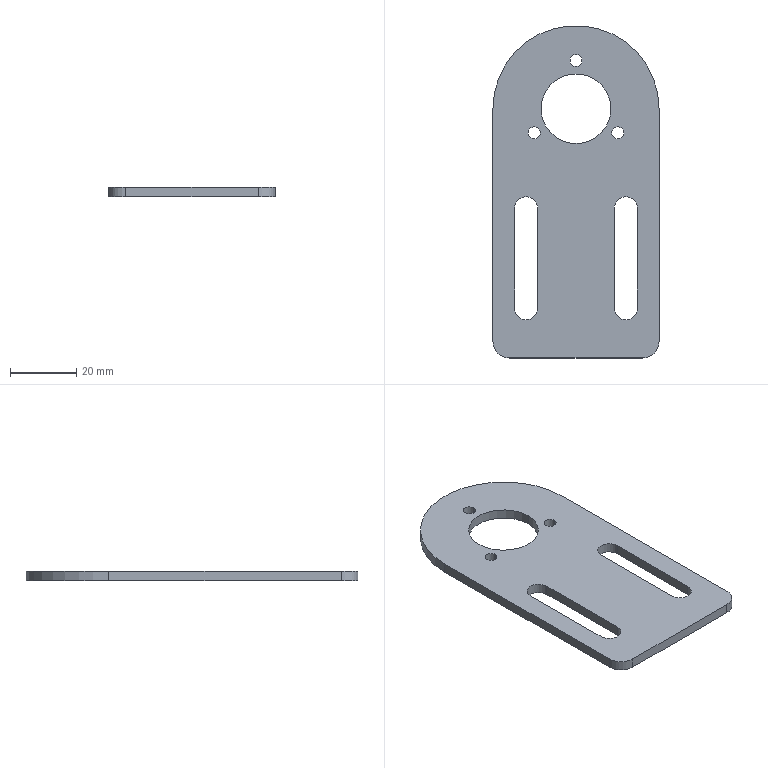Part | SolidWorks | features ICE 2, Fillet 1, FlatPattern 1, HoleWzd 1, SMBaseFlange 1, SheetMetal 1 | 1 solid | 24 faces | box 50 x 100 x 3 mm | volume 11541 mm3 | cylinder 15 | plane 9 | commonest cylinder face diameters 3.6 x6 7 x4 10 x2 21 x2 50 x1
STEP:
#1=CARTESIAN_POINT('',(23.2,89.5,-3.));
#2=VERTEX_POINT('',#1);
#3=CARTESIAN_POINT('',(26.8,89.5,-3.));
#4=VERTEX_POINT('',#3);
#5=CARTESIAN_POINT('',(25.,89.5,-3.));
#6=DIRECTION('',(0.,0.,1.));
#7=DIRECTION('',(1.,0.,0.));
#8=AXIS2_PLACEMENT_3D('',#5,#6,#7);
#9=CIRCLE('',#8,1.8);
#10=EDGE_CURVE('',#2,#4,#9,.T.);
#11=ORIENTED_EDGE('',*,*,#10,.F.);
#12=CARTESIAN_POINT('',(23.2,89.5,0.));
#13=VERTEX_POINT('',#12);
#14=CARTESIAN_POINT('',(23.2,89.5,0.));
#15=DIRECTION('',(0.,0.,1.));
#16=VECTOR('',#15,1000.);
#17=LINE('',#14,#16);
#18=EDGE_CURVE('',#2,#13,#17,.T.);
#19=ORIENTED_EDGE('',*,*,#18,.T.);
#20=CARTESIAN_POINT('',(26.8,89.5,0.));
#21=VERTEX_POINT('',#20);
#22=CARTESIAN_POINT('',(25.,89.5,0.));
#23=DIRECTION('',(0.,0.,1.));
#24=DIRECTION('',(1.,0.,0.));
#25=AXIS2_PLACEMENT_3D('',#22,#23,#24);
#26=CIRCLE('',#25,1.8);
#27=EDGE_CURVE('',#13,#21,#26,.T.);
#28=ORIENTED_EDGE('',*,*,#27,.T.);
#29=CARTESIAN_POINT('',(26.8,89.5,0.));
#30=DIRECTION('',(0.,0.,1.));
#31=VECTOR('',#30,1000.);
#32=LINE('',#29,#31);
#33=EDGE_CURVE('',#4,#21,#32,.T.);
#34=ORIENTED_EDGE('',*,*,#33,.F.);
#35=EDGE_LOOP('',(#11,#19,#28,#34));
#36=FACE_OUTER_BOUND('',#35,.T.);
#37=CARTESIAN_POINT('',(25.,89.5,0.));
#38=DIRECTION('',(0.,0.,1.));
#39=DIRECTION('',(1.,0.,0.));
#40=AXIS2_PLACEMENT_3D('',#37,#38,#39);
#41=CYLINDRICAL_SURFACE('',#40,1.8);
#42=ADVANCED_FACE('',(#36),#41,.F.);
#43=CARTESIAN_POINT('',(10.643,67.75,-3.));
#44=VERTEX_POINT('',#43);
#45=CARTESIAN_POINT('',(14.243,67.75,-3.));
#46=VERTEX_POINT('',#45);
#47=CARTESIAN_POINT('',(12.443,67.75,-3.));
#48=DIRECTION('',(0.,0.,1.));
#49=DIRECTION('',(1.,0.,0.));
#50=AXIS2_PLACEMENT_3D('',#47,#48,#49);
#51=CIRCLE('',#50,1.8);
#52=EDGE_CURVE('',#44,#46,#51,.T.);
#53=ORIENTED_EDGE('',*,*,#52,.F.);
#54=CARTESIAN_POINT('',(10.643,67.75,0.));
#55=VERTEX_POINT('',#54);
#56=CARTESIAN_POINT('',(10.643,67.75,0.));
#57=DIRECTION('',(0.,0.,1.));
#58=VECTOR('',#57,1000.);
#59=LINE('',#56,#58);
#60=EDGE_CURVE('',#44,#55,#59,.T.);
#61=ORIENTED_EDGE('',*,*,#60,.T.);
#62=CARTESIAN_POINT('',(14.243,67.75,0.));
#63=VERTEX_POINT('',#62);
#64=CARTESIAN_POINT('',(12.443,67.75,0.));
#65=DIRECTION('',(0.,0.,1.));
#66=DIRECTION('',(1.,0.,0.));
#67=AXIS2_PLACEMENT_3D('',#64,#65,#66);
#68=CIRCLE('',#67,1.8);
#69=EDGE_CURVE('',#55,#63,#68,.T.);
#70=ORIENTED_EDGE('',*,*,#69,.T.);
#71=CARTESIAN_POINT('',(14.243,67.75,0.));
#72=DIRECTION('',(0.,0.,1.));
#73=VECTOR('',#72,1000.);
#74=LINE('',#71,#73);
#75=EDGE_CURVE('',#46,#63,#74,.T.);
#76=ORIENTED_EDGE('',*,*,#75,.F.);
#77=EDGE_LOOP('',(#53,#61,#70,#76));
#78=FACE_OUTER_BOUND('',#77,.T.);
#79=CARTESIAN_POINT('',(12.443,67.75,0.));
#80=DIRECTION('',(0.,0.,1.));
#81=DIRECTION('',(1.,0.,0.));
#82=AXIS2_PLACEMENT_3D('',#79,#80,#81);
#83=CYLINDRICAL_SURFACE('',#82,1.8);
#84=ADVANCED_FACE('',(#78),#83,.F.);
#85=CARTESIAN_POINT('',(35.757,67.75,-3.));
#86=VERTEX_POINT('',#85);
#87=CARTESIAN_POINT('',(39.357,67.75,-3.));
#88=VERTEX_POINT('',#87);
#89=CARTESIAN_POINT('',(37.557,67.75,-3.));
#90=DIRECTION('',(0.,0.,1.));
#91=DIRECTION('',(1.,0.,0.));
#92=AXIS2_PLACEMENT_3D('',#89,#90,#91);
#93=CIRCLE('',#92,1.8);
#94=EDGE_CURVE('',#86,#88,#93,.T.);
#95=ORIENTED_EDGE('',*,*,#94,.F.);
#96=CARTESIAN_POINT('',(35.757,67.75,0.));
#97=VERTEX_POINT('',#96);
#98=CARTESIAN_POINT('',(35.757,67.75,0.));
#99=DIRECTION('',(0.,0.,1.));
#100=VECTOR('',#99,1000.);
#101=LINE('',#98,#100);
#102=EDGE_CURVE('',#86,#97,#101,.T.);
#103=ORIENTED_EDGE('',*,*,#102,.T.);
#104=CARTESIAN_POINT('',(39.357,67.75,0.));
#105=VERTEX_POINT('',#104);
#106=CARTESIAN_POINT('',(37.557,67.75,0.));
#107=DIRECTION('',(0.,0.,1.));
#108=DIRECTION('',(1.,0.,0.));
#109=AXIS2_PLACEMENT_3D('',#106,#107,#108);
#110=CIRCLE('',#109,1.8);
#111=EDGE_CURVE('',#97,#105,#110,.T.);
#112=ORIENTED_EDGE('',*,*,#111,.T.);
#113=CARTESIAN_POINT('',(39.357,67.75,0.));
#114=DIRECTION('',(0.,0.,1.));
#115=VECTOR('',#114,1000.);
#116=LINE('',#113,#115);
#117=EDGE_CURVE('',#88,#105,#116,.T.);
#118=ORIENTED_EDGE('',*,*,#117,.F.);
#119=EDGE_LOOP('',(#95,#103,#112,#118));
#120=FACE_OUTER_BOUND('',#119,.T.);
#121=CARTESIAN_POINT('',(37.557,67.75,0.));
#122=DIRECTION('',(0.,0.,1.));
#123=DIRECTION('',(1.,0.,0.));
#124=AXIS2_PLACEMENT_3D('',#121,#122,#123);
#125=CYLINDRICAL_SURFACE('',#124,1.8);
#126=ADVANCED_FACE('',(#120),#125,.F.);
#127=CARTESIAN_POINT('',(14.5,75.,-3.));
#128=VERTEX_POINT('',#127);
#129=CARTESIAN_POINT('',(35.5,75.,-3.));
#130=VERTEX_POINT('',#129);
#131=CARTESIAN_POINT('',(25.,75.,-3.));
#132=DIRECTION('',(0.,0.,1.));
#133=DIRECTION('',(1.,0.,0.));
#134=AXIS2_PLACEMENT_3D('',#131,#132,#133);
#135=CIRCLE('',#134,10.5);
#136=EDGE_CURVE('',#128,#130,#135,.T.);
#137=ORIENTED_EDGE('',*,*,#136,.F.);
#138=CARTESIAN_POINT('',(14.5,75.,0.));
#139=VERTEX_POINT('',#138);
#140=CARTESIAN_POINT('',(14.5,75.,-10.));
#141=DIRECTION('',(0.,0.,1.));
#142=VECTOR('',#141,1000.);
#143=LINE('',#140,#142);
#144=EDGE_CURVE('',#128,#139,#143,.T.);
#145=ORIENTED_EDGE('',*,*,#144,.T.);
#146=CARTESIAN_POINT('',(35.5,75.,0.));
#147=VERTEX_POINT('',#146);
#148=CARTESIAN_POINT('',(25.,75.,0.));
#149=DIRECTION('',(0.,0.,1.));
#150=DIRECTION('',(1.,0.,0.));
#151=AXIS2_PLACEMENT_3D('',#148,#149,#150);
#152=CIRCLE('',#151,10.5);
#153=EDGE_CURVE('',#139,#147,#152,.T.);
#154=ORIENTED_EDGE('',*,*,#153,.T.);
#155=CARTESIAN_POINT('',(35.5,75.,-10.));
#156=DIRECTION('',(0.,0.,1.));
#157=VECTOR('',#156,1000.);
#158=LINE('',#155,#157);
#159=EDGE_CURVE('',#130,#147,#158,.T.);
#160=ORIENTED_EDGE('',*,*,#159,.F.);
#161=EDGE_LOOP('',(#137,#145,#154,#160));
#162=FACE_OUTER_BOUND('',#161,.T.);
#163=CARTESIAN_POINT('',(25.,75.,-10.));
#164=DIRECTION('',(0.,0.,1.));
#165=DIRECTION('',(1.,0.,0.));
#166=AXIS2_PLACEMENT_3D('',#163,#164,#165);
#167=CYLINDRICAL_SURFACE('',#166,10.5);
#168=ADVANCED_FACE('',(#162),#167,.F.);
#169=CARTESIAN_POINT('',(0.,75.,-3.));
#170=VERTEX_POINT('',#169);
#171=CARTESIAN_POINT('',(0.,5.,-3.));
#172=VERTEX_POINT('',#171);
#173=CARTESIAN_POINT('',(0.,0.,-3.));
#174=DIRECTION('',(0.,-1.,0.));
#175=VECTOR('',#174,1000.);
#176=LINE('',#173,#175);
#177=EDGE_CURVE('',#170,#172,#176,.T.);
#178=ORIENTED_EDGE('',*,*,#177,.T.);
#179=CARTESIAN_POINT('',(0.,5.,0.));
#180=VERTEX_POINT('',#179);
#181=CARTESIAN_POINT('',(0.,5.,-3.));
#182=DIRECTION('',(0.,0.,1.));
#183=VECTOR('',#182,1000.);
#184=LINE('',#181,#183);
#185=EDGE_CURVE('',#172,#180,#184,.T.);
#186=ORIENTED_EDGE('',*,*,#185,.T.);
#187=CARTESIAN_POINT('',(0.,75.,0.));
#188=VERTEX_POINT('',#187);
#189=CARTESIAN_POINT('',(0.,0.,0.));
#190=DIRECTION('',(0.,-1.,0.));
#191=VECTOR('',#190,1000.);
#192=LINE('',#189,#191);
#193=EDGE_CURVE('',#188,#180,#192,.T.);
#194=ORIENTED_EDGE('',*,*,#193,.F.);
#195=CARTESIAN_POINT('',(0.,75.,-3.));
#196=DIRECTION('',(0.,0.,1.));
#197=VECTOR('',#196,1000.);
#198=LINE('',#195,#197);
#199=EDGE_CURVE('',#170,#188,#198,.T.);
#200=ORIENTED_EDGE('',*,*,#199,.F.);
#201=EDGE_LOOP('',(#178,#186,#194,#200));
#202=FACE_OUTER_BOUND('',#201,.T.);
#203=CARTESIAN_POINT('',(0.,0.,-3.));
#204=DIRECTION('',(-1.,0.,0.));
#205=DIRECTION('',(0.,-1.,0.));
#206=AXIS2_PLACEMENT_3D('',#203,#204,#205);
#207=PLANE('',#206);
#208=ADVANCED_FACE('',(#202),#207,.T.);
#209=CARTESIAN_POINT('',(50.,75.,0.));
#210=VERTEX_POINT('',#209);
#211=CARTESIAN_POINT('',(25.,75.,0.));
#212=DIRECTION('',(0.,0.,1.));
#213=DIRECTION('',(1.,0.,0.));
#214=AXIS2_PLACEMENT_3D('',#211,#212,#213);
#215=CIRCLE('',#214,25.);
#216=EDGE_CURVE('',#210,#188,#215,.T.);
#217=ORIENTED_EDGE('',*,*,#216,.F.);
#218=CARTESIAN_POINT('',(50.,75.,-3.));
#219=VERTEX_POINT('',#218);
#220=CARTESIAN_POINT('',(50.,75.,-3.));
#221=DIRECTION('',(0.,0.,1.));
#222=VECTOR('',#221,1000.);
#223=LINE('',#220,#222);
#224=EDGE_CURVE('',#219,#210,#223,.T.);
#225=ORIENTED_EDGE('',*,*,#224,.F.);
#226=CARTESIAN_POINT('',(25.,75.,-3.));
#227=DIRECTION('',(0.,0.,1.));
#228=DIRECTION('',(1.,0.,0.));
#229=AXIS2_PLACEMENT_3D('',#226,#227,#228);
#230=CIRCLE('',#229,25.);
#231=EDGE_CURVE('',#219,#170,#230,.T.);
#232=ORIENTED_EDGE('',*,*,#231,.T.);
#233=ORIENTED_EDGE('',*,*,#199,.T.);
#234=EDGE_LOOP('',(#217,#225,#232,#233));
#235=FACE_OUTER_BOUND('',#234,.T.);
#236=CARTESIAN_POINT('',(25.,75.,-3.));
#237=DIRECTION('',(0.,0.,1.));
#238=DIRECTION('',(1.,0.,0.));
#239=AXIS2_PLACEMENT_3D('',#236,#237,#238);
#240=CYLINDRICAL_SURFACE('',#239,25.);
#241=ADVANCED_FACE('',(#235),#240,.T.);
#242=CARTESIAN_POINT('',(50.,5.,0.));
#243=VERTEX_POINT('',#242);
#244=CARTESIAN_POINT('',(50.,0.,0.));
#245=DIRECTION('',(0.,1.,0.));
#246=VECTOR('',#245,1000.);
#247=LINE('',#244,#246);
#248=EDGE_CURVE('',#243,#210,#247,.T.);
#249=ORIENTED_EDGE('',*,*,#248,.F.);
#250=CARTESIAN_POINT('',(50.,5.,-3.));
#251=VERTEX_POINT('',#250);
#252=CARTESIAN_POINT('',(50.,5.,-3.));
#253=DIRECTION('',(0.,0.,-1.));
#254=VECTOR('',#253,1000.);
#255=LINE('',#252,#254);
#256=EDGE_CURVE('',#243,#251,#255,.T.);
#257=ORIENTED_EDGE('',*,*,#256,.T.);
#258=CARTESIAN_POINT('',(50.,0.,-3.));
#259=DIRECTION('',(0.,1.,0.));
#260=VECTOR('',#259,1000.);
#261=LINE('',#258,#260);
#262=EDGE_CURVE('',#251,#219,#261,.T.);
#263=ORIENTED_EDGE('',*,*,#262,.T.);
#264=ORIENTED_EDGE('',*,*,#224,.T.);
#265=EDGE_LOOP('',(#249,#257,#263,#264));
#266=FACE_OUTER_BOUND('',#265,.T.);
#267=CARTESIAN_POINT('',(50.,0.,-3.));
#268=DIRECTION('',(1.,0.,0.));
#269=DIRECTION('',(0.,1.,0.));
#270=AXIS2_PLACEMENT_3D('',#267,#268,#269);
#271=PLANE('',#270);
#272=ADVANCED_FACE('',(#266),#271,.T.);
#273=CARTESIAN_POINT('',(5.,0.,-3.));
#274=VERTEX_POINT('',#273);
#275=CARTESIAN_POINT('',(45.,0.,-3.));
#276=VERTEX_POINT('',#275);
#277=CARTESIAN_POINT('',(0.,0.,-3.));
#278=DIRECTION('',(1.,0.,0.));
#279=VECTOR('',#278,1000.);
#280=LINE('',#277,#279);
#281=EDGE_CURVE('',#274,#276,#280,.T.);
#282=ORIENTED_EDGE('',*,*,#281,.T.);
#283=CARTESIAN_POINT('',(45.,0.,0.));
#284=VERTEX_POINT('',#283);
#285=CARTESIAN_POINT('',(45.,0.,-3.));
#286=DIRECTION('',(0.,0.,1.));
#287=VECTOR('',#286,1000.);
#288=LINE('',#285,#287);
#289=EDGE_CURVE('',#276,#284,#288,.T.);
#290=ORIENTED_EDGE('',*,*,#289,.T.);
#291=CARTESIAN_POINT('',(5.,0.,0.));
#292=VERTEX_POINT('',#291);
#293=CARTESIAN_POINT('',(0.,0.,0.));
#294=DIRECTION('',(1.,0.,0.));
#295=VECTOR('',#294,1000.);
#296=LINE('',#293,#295);
#297=EDGE_CURVE('',#292,#284,#296,.T.);
#298=ORIENTED_EDGE('',*,*,#297,.F.);
#299=CARTESIAN_POINT('',(5.,0.,-3.));
#300=DIRECTION('',(0.,0.,-1.));
#301=VECTOR('',#300,1000.);
#302=LINE('',#299,#301);
#303=EDGE_CURVE('',#292,#274,#302,.T.);
#304=ORIENTED_EDGE('',*,*,#303,.T.);
#305=EDGE_LOOP('',(#282,#290,#298,#304));
#306=FACE_OUTER_BOUND('',#305,.T.);
#307=CARTESIAN_POINT('',(0.,0.,-3.));
#308=DIRECTION('',(0.,-1.,0.));
#309=DIRECTION('',(1.,0.,0.));
#310=AXIS2_PLACEMENT_3D('',#307,#308,#309);
#311=PLANE('',#310);
#312=ADVANCED_FACE('',(#306),#311,.T.);
#313=CARTESIAN_POINT('',(13.5,15.,-3.));
#314=VERTEX_POINT('',#313);
#315=CARTESIAN_POINT('',(13.5,45.,-3.));
#316=VERTEX_POINT('',#315);
#317=CARTESIAN_POINT('',(13.5,75.,-3.));
#318=DIRECTION('',(0.,1.,0.));
#319=VECTOR('',#318,1000.);
#320=LINE('',#317,#319);
#321=EDGE_CURVE('',#314,#316,#320,.T.);
#322=ORIENTED_EDGE('',*,*,#321,.T.);
#323=CARTESIAN_POINT('',(6.5,45.,-3.));
#324=VERTEX_POINT('',#323);
#325=CARTESIAN_POINT('',(10.,45.,-3.));
#326=DIRECTION('',(0.,0.,1.));
#327=DIRECTION('',(1.,0.,0.));
#328=AXIS2_PLACEMENT_3D('',#325,#326,#327);
#329=CIRCLE('',#328,3.5);
#330=EDGE_CURVE('',#316,#324,#329,.T.);
#331=ORIENTED_EDGE('',*,*,#330,.T.);
#332=CARTESIAN_POINT('',(6.5,15.,-3.));
#333=VERTEX_POINT('',#332);
#334=CARTESIAN_POINT('',(6.5,75.,-3.));
#335=DIRECTION('',(0.,-1.,0.));
#336=VECTOR('',#335,1000.);
#337=LINE('',#334,#336);
#338=EDGE_CURVE('',#324,#333,#337,.T.);
#339=ORIENTED_EDGE('',*,*,#338,.T.);
#340=CARTESIAN_POINT('',(10.,15.,-3.));
#341=DIRECTION('',(0.,0.,1.));
#342=DIRECTION('',(1.,0.,0.));
#343=AXIS2_PLACEMENT_3D('',#340,#341,#342);
#344=CIRCLE('',#343,3.5);
#345=EDGE_CURVE('',#333,#314,#344,.T.);
#346=ORIENTED_EDGE('',*,*,#345,.T.);
#347=EDGE_LOOP('',(#322,#331,#339,#346));
#348=FACE_BOUND('',#347,.T.);
#349=CARTESIAN_POINT('',(43.5,15.,-3.));
#350=VERTEX_POINT('',#349);
#351=CARTESIAN_POINT('',(43.5,45.,-3.));
#352=VERTEX_POINT('',#351);
#353=CARTESIAN_POINT('',(43.5,75.,-3.));
#354=DIRECTION('',(0.,1.,0.));
#355=VECTOR('',#354,1000.);
#356=LINE('',#353,#355);
#357=EDGE_CURVE('',#350,#352,#356,.T.);
#358=ORIENTED_EDGE('',*,*,#357,.T.);
#359=CARTESIAN_POINT('',(36.5,45.,-3.));
#360=VERTEX_POINT('',#359);
#361=CARTESIAN_POINT('',(40.,45.,-3.));
#362=DIRECTION('',(0.,0.,1.));
#363=DIRECTION('',(1.,0.,0.));
#364=AXIS2_PLACEMENT_3D('',#361,#362,#363);
#365=CIRCLE('',#364,3.5);
#366=EDGE_CURVE('',#352,#360,#365,.T.);
#367=ORIENTED_EDGE('',*,*,#366,.T.);
#368=CARTESIAN_POINT('',(36.5,15.,-3.));
#369=VERTEX_POINT('',#368);
#370=CARTESIAN_POINT('',(36.5,75.,-3.));
#371=DIRECTION('',(0.,-1.,0.));
#372=VECTOR('',#371,1000.);
#373=LINE('',#370,#372);
#374=EDGE_CURVE('',#360,#369,#373,.T.);
#375=ORIENTED_EDGE('',*,*,#374,.T.);
#376=CARTESIAN_POINT('',(40.,15.,-3.));
#377=DIRECTION('',(0.,0.,1.));
#378=DIRECTION('',(1.,0.,0.));
#379=AXIS2_PLACEMENT_3D('',#376,#377,#378);
#380=CIRCLE('',#379,3.5);
#381=EDGE_CURVE('',#369,#350,#380,.T.);
#382=ORIENTED_EDGE('',*,*,#381,.T.);
#383=EDGE_LOOP('',(#358,#367,#375,#382));
#384=FACE_BOUND('',#383,.T.);
#385=CARTESIAN_POINT('',(25.,89.5,-3.));
#386=DIRECTION('',(0.,0.,1.));
#387=DIRECTION('',(1.,0.,0.));
#388=AXIS2_PLACEMENT_3D('',#385,#386,#387);
#389=CIRCLE('',#388,1.8);
#390=EDGE_CURVE('',#4,#2,#389,.T.);
#391=ORIENTED_EDGE('',*,*,#390,.T.);
#392=ORIENTED_EDGE('',*,*,#10,.T.);
#393=EDGE_LOOP('',(#391,#392));
#394=FACE_BOUND('',#393,.T.);
#395=CARTESIAN_POINT('',(12.443,67.75,-3.));
#396=DIRECTION('',(0.,0.,1.));
#397=DIRECTION('',(1.,0.,0.));
#398=AXIS2_PLACEMENT_3D('',#395,#396,#397);
#399=CIRCLE('',#398,1.8);
#400=EDGE_CURVE('',#46,#44,#399,.T.);
#401=ORIENTED_EDGE('',*,*,#400,.T.);
#402=ORIENTED_EDGE('',*,*,#52,.T.);
#403=EDGE_LOOP('',(#401,#402));
#404=FACE_BOUND('',#403,.T.);
#405=CARTESIAN_POINT('',(37.557,67.75,-3.));
#406=DIRECTION('',(0.,0.,1.));
#407=DIRECTION('',(1.,0.,0.));
#408=AXIS2_PLACEMENT_3D('',#405,#406,#407);
#409=CIRCLE('',#408,1.8);
#410=EDGE_CURVE('',#88,#86,#409,.T.);
#411=ORIENTED_EDGE('',*,*,#410,.T.);
#412=ORIENTED_EDGE('',*,*,#94,.T.);
#413=EDGE_LOOP('',(#411,#412));
#414=FACE_BOUND('',#413,.T.);
#415=CARTESIAN_POINT('',(25.,75.,-3.));
#416=DIRECTION('',(0.,0.,1.));
#417=DIRECTION('',(1.,0.,0.));
#418=AXIS2_PLACEMENT_3D('',#415,#416,#417);
#419=CIRCLE('',#418,10.5);
#420=EDGE_CURVE('',#130,#128,#419,.T.);
#421=ORIENTED_EDGE('',*,*,#420,.T.);
#422=ORIENTED_EDGE('',*,*,#136,.T.);
#423=EDGE_LOOP('',(#421,#422));
#424=FACE_BOUND('',#423,.T.);
#425=ORIENTED_EDGE('',*,*,#262,.F.);
#426=CARTESIAN_POINT('',(45.,5.,-3.));
#427=DIRECTION('',(0.,0.,-1.));
#428=DIRECTION('',(1.,0.,0.));
#429=AXIS2_PLACEMENT_3D('',#426,#427,#428);
#430=CIRCLE('',#429,5.);
#431=EDGE_CURVE('',#251,#276,#430,.T.);
#432=ORIENTED_EDGE('',*,*,#431,.T.);
#433=ORIENTED_EDGE('',*,*,#281,.F.);
#434=CARTESIAN_POINT('',(5.,5.,-3.));
#435=DIRECTION('',(0.,0.,-1.));
#436=DIRECTION('',(1.,0.,0.));
#437=AXIS2_PLACEMENT_3D('',#434,#435,#436);
#438=CIRCLE('',#437,5.);
#439=EDGE_CURVE('',#274,#172,#438,.T.);
#440=ORIENTED_EDGE('',*,*,#439,.T.);
#441=ORIENTED_EDGE('',*,*,#177,.F.);
#442=ORIENTED_EDGE('',*,*,#231,.F.);
#443=EDGE_LOOP('',(#425,#432,#433,#440,#441,#442));
#444=FACE_OUTER_BOUND('',#443,.T.);
#445=CARTESIAN_POINT('',(25.,75.,-3.));
#446=DIRECTION('',(0.,0.,1.));
#447=DIRECTION('',(1.,0.,0.));
#448=AXIS2_PLACEMENT_3D('',#445,#446,#447);
#449=PLANE('',#448);
#450=ADVANCED_FACE('',(#348,#384,#394,#404,#414,#424,#444),#449,.F.);
#451=CARTESIAN_POINT('',(13.5,45.,0.));
#452=VERTEX_POINT('',#451);
#453=CARTESIAN_POINT('',(6.5,45.,0.));
#454=VERTEX_POINT('',#453);
#455=CARTESIAN_POINT('',(10.,45.,0.));
#456=DIRECTION('',(0.,0.,1.));
#457=DIRECTION('',(1.,0.,0.));
#458=AXIS2_PLACEMENT_3D('',#455,#456,#457);
#459=CIRCLE('',#458,3.5);
#460=EDGE_CURVE('',#452,#454,#459,.T.);
#461=ORIENTED_EDGE('',*,*,#460,.F.);
#462=CARTESIAN_POINT('',(13.5,15.,0.));
#463=VERTEX_POINT('',#462);
#464=CARTESIAN_POINT('',(13.5,45.,0.));
#465=DIRECTION('',(0.,1.,0.));
#466=VECTOR('',#465,1000.);
#467=LINE('',#464,#466);
#468=EDGE_CURVE('',#463,#452,#467,.T.);
#469=ORIENTED_EDGE('',*,*,#468,.F.);
#470=CARTESIAN_POINT('',(6.5,15.,0.));
#471=VERTEX_POINT('',#470);
#472=CARTESIAN_POINT('',(10.,15.,0.));
#473=DIRECTION('',(0.,0.,1.));
#474=DIRECTION('',(1.,0.,0.));
#475=AXIS2_PLACEMENT_3D('',#472,#473,#474);
#476=CIRCLE('',#475,3.5);
#477=EDGE_CURVE('',#471,#463,#476,.T.);
#478=ORIENTED_EDGE('',*,*,#477,.F.);
#479=CARTESIAN_POINT('',(6.5,45.,0.));
#480=DIRECTION('',(0.,-1.,0.));
#481=VECTOR('',#480,1000.);
#482=LINE('',#479,#481);
#483=EDGE_CURVE('',#454,#471,#482,.T.);
#484=ORIENTED_EDGE('',*,*,#483,.F.);
#485=EDGE_LOOP('',(#461,#469,#478,#484));
#486=FACE_BOUND('',#485,.T.);
#487=CARTESIAN_POINT('',(43.5,45.,0.));
#488=VERTEX_POINT('',#487);
#489=CARTESIAN_POINT('',(36.5,45.,0.));
#490=VERTEX_POINT('',#489);
#491=CARTESIAN_POINT('',(40.,45.,0.));
#492=DIRECTION('',(0.,0.,1.));
#493=DIRECTION('',(-1.,0.,0.));
#494=AXIS2_PLACEMENT_3D('',#491,#492,#493);
#495=CIRCLE('',#494,3.5);
#496=EDGE_CURVE('',#488,#490,#495,.T.);
#497=ORIENTED_EDGE('',*,*,#496,.F.);
#498=CARTESIAN_POINT('',(43.5,15.,0.));
#499=VERTEX_POINT('',#498);
#500=CARTESIAN_POINT('',(43.5,45.,0.));
#501=DIRECTION('',(0.,1.,0.));
#502=VECTOR('',#501,1000.);
#503=LINE('',#500,#502);
#504=EDGE_CURVE('',#499,#488,#503,.T.);
#505=ORIENTED_EDGE('',*,*,#504,.F.);
#506=CARTESIAN_POINT('',(36.5,15.,0.));
#507=VERTEX_POINT('',#506);
#508=CARTESIAN_POINT('',(40.,15.,0.));
#509=DIRECTION('',(0.,0.,1.));
#510=DIRECTION('',(-1.,0.,0.));
#511=AXIS2_PLACEMENT_3D('',#508,#509,#510);
#512=CIRCLE('',#511,3.5);
#513=EDGE_CURVE('',#507,#499,#512,.T.);
#514=ORIENTED_EDGE('',*,*,#513,.F.);
#515=CARTESIAN_POINT('',(36.5,45.,0.));
#516=DIRECTION('',(0.,-1.,0.));
#517=VECTOR('',#516,1000.);
#518=LINE('',#515,#517);
#519=EDGE_CURVE('',#490,#507,#518,.T.);
#520=ORIENTED_EDGE('',*,*,#519,.F.);
#521=EDGE_LOOP('',(#497,#505,#514,#520));
#522=FACE_BOUND('',#521,.T.);
#523=CARTESIAN_POINT('',(25.,89.5,0.));
#524=DIRECTION('',(0.,0.,1.));
#525=DIRECTION('',(1.,0.,0.));
#526=AXIS2_PLACEMENT_3D('',#523,#524,#525);
#527=CIRCLE('',#526,1.8);
#528=EDGE_CURVE('',#21,#13,#527,.T.);
#529=ORIENTED_EDGE('',*,*,#528,.F.);
#530=ORIENTED_EDGE('',*,*,#27,.F.);
#531=EDGE_LOOP('',(#529,#530));
#532=FACE_BOUND('',#531,.T.);
#533=CARTESIAN_POINT('',(12.443,67.75,0.));
#534=DIRECTION('',(0.,0.,1.));
#535=DIRECTION('',(1.,0.,0.));
#536=AXIS2_PLACEMENT_3D('',#533,#534,#535);
#537=CIRCLE('',#536,1.8);
#538=EDGE_CURVE('',#63,#55,#537,.T.);
#539=ORIENTED_EDGE('',*,*,#538,.F.);
#540=ORIENTED_EDGE('',*,*,#69,.F.);
#541=EDGE_LOOP('',(#539,#540));
#542=FACE_BOUND('',#541,.T.);
#543=CARTESIAN_POINT('',(37.557,67.75,0.));
#544=DIRECTION('',(0.,0.,1.));
#545=DIRECTION('',(1.,0.,0.));
#546=AXIS2_PLACEMENT_3D('',#543,#544,#545);
#547=CIRCLE('',#546,1.8);
#548=EDGE_CURVE('',#105,#97,#547,.T.);
#549=ORIENTED_EDGE('',*,*,#548,.F.);
#550=ORIENTED_EDGE('',*,*,#111,.F.);
#551=EDGE_LOOP('',(#549,#550));
#552=FACE_BOUND('',#551,.T.);
#553=CARTESIAN_POINT('',(25.,75.,0.));
#554=DIRECTION('',(0.,0.,1.));
#555=DIRECTION('',(1.,0.,0.));
#556=AXIS2_PLACEMENT_3D('',#553,#554,#555);
#557=CIRCLE('',#556,10.5);
#558=EDGE_CURVE('',#147,#139,#557,.T.);
#559=ORIENTED_EDGE('',*,*,#558,.F.);
#560=ORIENTED_EDGE('',*,*,#153,.F.);
#561=EDGE_LOOP('',(#559,#560));
#562=FACE_BOUND('',#561,.T.);
#563=ORIENTED_EDGE('',*,*,#297,.T.);
#564=CARTESIAN_POINT('',(45.,5.,0.));
#565=DIRECTION('',(0.,0.,1.));
#566=DIRECTION('',(1.,0.,0.));
#567=AXIS2_PLACEMENT_3D('',#564,#565,#566);
#568=CIRCLE('',#567,5.);
#569=EDGE_CURVE('',#284,#243,#568,.T.);
#570=ORIENTED_EDGE('',*,*,#569,.T.);
#571=ORIENTED_EDGE('',*,*,#248,.T.);
#572=ORIENTED_EDGE('',*,*,#216,.T.);
#573=ORIENTED_EDGE('',*,*,#193,.T.);
#574=CARTESIAN_POINT('',(5.,5.,0.));
#575=DIRECTION('',(0.,0.,1.));
#576=DIRECTION('',(1.,0.,0.));
#577=AXIS2_PLACEMENT_3D('',#574,#575,#576);
#578=CIRCLE('',#577,5.);
#579=EDGE_CURVE('',#180,#292,#578,.T.);
#580=ORIENTED_EDGE('',*,*,#579,.T.);
#581=EDGE_LOOP('',(#563,#570,#571,#572,#573,#580));
#582=FACE_OUTER_BOUND('',#581,.T.);
#583=CARTESIAN_POINT('',(25.,75.,0.));
#584=DIRECTION('',(0.,0.,1.));
#585=DIRECTION('',(1.,0.,0.));
#586=AXIS2_PLACEMENT_3D('',#583,#584,#585);
#587=PLANE('',#586);
#588=ADVANCED_FACE('',(#486,#522,#532,#542,#552,#562,#582),#587,.T.);
#589=ORIENTED_EDGE('',*,*,#144,.F.);
#590=ORIENTED_EDGE('',*,*,#420,.F.);
#591=ORIENTED_EDGE('',*,*,#159,.T.);
#592=ORIENTED_EDGE('',*,*,#558,.T.);
#593=EDGE_LOOP('',(#589,#590,#591,#592));
#594=FACE_OUTER_BOUND('',#593,.T.);
#595=CARTESIAN_POINT('',(25.,75.,-10.));
#596=DIRECTION('',(0.,0.,1.));
#597=DIRECTION('',(1.,0.,0.));
#598=AXIS2_PLACEMENT_3D('',#595,#596,#597);
#599=CYLINDRICAL_SURFACE('',#598,10.5);
#600=ADVANCED_FACE('',(#594),#599,.F.);
#601=ORIENTED_EDGE('',*,*,#102,.F.);
#602=ORIENTED_EDGE('',*,*,#410,.F.);
#603=ORIENTED_EDGE('',*,*,#117,.T.);
#604=ORIENTED_EDGE('',*,*,#548,.T.);
#605=EDGE_LOOP('',(#601,#602,#603,#604));
#606=FACE_OUTER_BOUND('',#605,.T.);
#607=CARTESIAN_POINT('',(37.557,67.75,0.));
#608=DIRECTION('',(0.,0.,1.));
#609=DIRECTION('',(1.,0.,0.));
#610=AXIS2_PLACEMENT_3D('',#607,#608,#609);
#611=CYLINDRICAL_SURFACE('',#610,1.8);
#612=ADVANCED_FACE('',(#606),#611,.F.);
#613=ORIENTED_EDGE('',*,*,#60,.F.);
#614=ORIENTED_EDGE('',*,*,#400,.F.);
#615=ORIENTED_EDGE('',*,*,#75,.T.);
#616=ORIENTED_EDGE('',*,*,#538,.T.);
#617=EDGE_LOOP('',(#613,#614,#615,#616));
#618=FACE_OUTER_BOUND('',#617,.T.);
#619=CARTESIAN_POINT('',(12.443,67.75,0.));
#620=DIRECTION('',(0.,0.,1.));
#621=DIRECTION('',(1.,0.,0.));
#622=AXIS2_PLACEMENT_3D('',#619,#620,#621);
#623=CYLINDRICAL_SURFACE('',#622,1.8);
#624=ADVANCED_FACE('',(#618),#623,.F.);
#625=ORIENTED_EDGE('',*,*,#18,.F.);
#626=ORIENTED_EDGE('',*,*,#390,.F.);
#627=ORIENTED_EDGE('',*,*,#33,.T.);
#628=ORIENTED_EDGE('',*,*,#528,.T.);
#629=EDGE_LOOP('',(#625,#626,#627,#628));
#630=FACE_OUTER_BOUND('',#629,.T.);
#631=CARTESIAN_POINT('',(25.,89.5,0.));
#632=DIRECTION('',(0.,0.,1.));
#633=DIRECTION('',(1.,0.,0.));
#634=AXIS2_PLACEMENT_3D('',#631,#632,#633);
#635=CYLINDRICAL_SURFACE('',#634,1.8);
#636=ADVANCED_FACE('',(#630),#635,.F.);
#637=CARTESIAN_POINT('',(43.5,45.,-10.));
#638=DIRECTION('',(0.,0.,1.));
#639=VECTOR('',#638,1000.);
#640=LINE('',#637,#639);
#641=EDGE_CURVE('',#352,#488,#640,.T.);
#642=ORIENTED_EDGE('',*,*,#641,.T.);
#643=ORIENTED_EDGE('',*,*,#496,.T.);
#644=CARTESIAN_POINT('',(36.5,45.,-10.));
#645=DIRECTION('',(0.,0.,1.));
#646=VECTOR('',#645,1000.);
#647=LINE('',#644,#646);
#648=EDGE_CURVE('',#360,#490,#647,.T.);
#649=ORIENTED_EDGE('',*,*,#648,.F.);
#650=ORIENTED_EDGE('',*,*,#366,.F.);
#651=EDGE_LOOP('',(#642,#643,#649,#650));
#652=FACE_OUTER_BOUND('',#651,.T.);
#653=CARTESIAN_POINT('',(40.,45.,-10.));
#654=DIRECTION('',(0.,0.,1.));
#655=DIRECTION('',(1.,0.,0.));
#656=AXIS2_PLACEMENT_3D('',#653,#654,#655);
#657=CYLINDRICAL_SURFACE('',#656,3.5);
#658=ADVANCED_FACE('',(#652),#657,.F.);
#659=CARTESIAN_POINT('',(43.5,15.,-10.));
#660=DIRECTION('',(0.,0.,1.));
#661=VECTOR('',#660,1000.);
#662=LINE('',#659,#661);
#663=EDGE_CURVE('',#350,#499,#662,.T.);
#664=ORIENTED_EDGE('',*,*,#663,.T.);
#665=ORIENTED_EDGE('',*,*,#504,.T.);
#666=ORIENTED_EDGE('',*,*,#641,.F.);
#667=ORIENTED_EDGE('',*,*,#357,.F.);
#668=EDGE_LOOP('',(#664,#665,#666,#667));
#669=FACE_OUTER_BOUND('',#668,.T.);
#670=CARTESIAN_POINT('',(43.5,45.,-10.));
#671=DIRECTION('',(1.,0.,0.));
#672=DIRECTION('',(0.,0.,-1.));
#673=AXIS2_PLACEMENT_3D('',#670,#671,#672);
#674=PLANE('',#673);
#675=ADVANCED_FACE('',(#669),#674,.F.);
#676=CARTESIAN_POINT('',(36.5,15.,-10.));
#677=DIRECTION('',(0.,0.,1.));
#678=VECTOR('',#677,1000.);
#679=LINE('',#676,#678);
#680=EDGE_CURVE('',#369,#507,#679,.T.);
#681=ORIENTED_EDGE('',*,*,#680,.T.);
#682=ORIENTED_EDGE('',*,*,#513,.T.);
#683=ORIENTED_EDGE('',*,*,#663,.F.);
#684=ORIENTED_EDGE('',*,*,#381,.F.);
#685=EDGE_LOOP('',(#681,#682,#683,#684));
#686=FACE_OUTER_BOUND('',#685,.T.);
#687=CARTESIAN_POINT('',(40.,15.,-10.));
#688=DIRECTION('',(0.,0.,1.));
#689=DIRECTION('',(1.,0.,0.));
#690=AXIS2_PLACEMENT_3D('',#687,#688,#689);
#691=CYLINDRICAL_SURFACE('',#690,3.5);
#692=ADVANCED_FACE('',(#686),#691,.F.);
#693=ORIENTED_EDGE('',*,*,#648,.T.);
#694=ORIENTED_EDGE('',*,*,#519,.T.);
#695=ORIENTED_EDGE('',*,*,#680,.F.);
#696=ORIENTED_EDGE('',*,*,#374,.F.);
#697=EDGE_LOOP('',(#693,#694,#695,#696));
#698=FACE_OUTER_BOUND('',#697,.T.);
#699=CARTESIAN_POINT('',(36.5,45.,-10.));
#700=DIRECTION('',(-1.,0.,0.));
#701=DIRECTION('',(0.,0.,1.));
#702=AXIS2_PLACEMENT_3D('',#699,#700,#701);
#703=PLANE('',#702);
#704=ADVANCED_FACE('',(#698),#703,.F.);
#705=CARTESIAN_POINT('',(13.5,45.,-10.));
#706=DIRECTION('',(0.,0.,1.));
#707=VECTOR('',#706,1000.);
#708=LINE('',#705,#707);
#709=EDGE_CURVE('',#316,#452,#708,.T.);
#710=ORIENTED_EDGE('',*,*,#709,.T.);
#711=ORIENTED_EDGE('',*,*,#460,.T.);
#712=CARTESIAN_POINT('',(6.5,45.,-10.));
#713=DIRECTION('',(0.,0.,1.));
#714=VECTOR('',#713,1000.);
#715=LINE('',#712,#714);
#716=EDGE_CURVE('',#324,#454,#715,.T.);
#717=ORIENTED_EDGE('',*,*,#716,.F.);
#718=ORIENTED_EDGE('',*,*,#330,.F.);
#719=EDGE_LOOP('',(#710,#711,#717,#718));
#720=FACE_OUTER_BOUND('',#719,.T.);
#721=CARTESIAN_POINT('',(10.,45.,-10.));
#722=DIRECTION('',(0.,0.,1.));
#723=DIRECTION('',(1.,0.,0.));
#724=AXIS2_PLACEMENT_3D('',#721,#722,#723);
#725=CYLINDRICAL_SURFACE('',#724,3.5);
#726=ADVANCED_FACE('',(#720),#725,.F.);
#727=CARTESIAN_POINT('',(13.5,15.,-10.));
#728=DIRECTION('',(0.,0.,1.));
#729=VECTOR('',#728,1000.);
#730=LINE('',#727,#729);
#731=EDGE_CURVE('',#314,#463,#730,.T.);
#732=ORIENTED_EDGE('',*,*,#731,.T.);
#733=ORIENTED_EDGE('',*,*,#468,.T.);
#734=ORIENTED_EDGE('',*,*,#709,.F.);
#735=ORIENTED_EDGE('',*,*,#321,.F.);
#736=EDGE_LOOP('',(#732,#733,#734,#735));
#737=FACE_OUTER_BOUND('',#736,.T.);
#738=CARTESIAN_POINT('',(13.5,45.,-10.));
#739=DIRECTION('',(1.,0.,0.));
#740=DIRECTION('',(0.,1.,0.));
#741=AXIS2_PLACEMENT_3D('',#738,#739,#740);
#742=PLANE('',#741);
#743=ADVANCED_FACE('',(#737),#742,.F.);
#744=CARTESIAN_POINT('',(6.5,15.,-10.));
#745=DIRECTION('',(0.,0.,1.));
#746=VECTOR('',#745,1000.);
#747=LINE('',#744,#746);
#748=EDGE_CURVE('',#333,#471,#747,.T.);
#749=ORIENTED_EDGE('',*,*,#748,.T.);
#750=ORIENTED_EDGE('',*,*,#477,.T.);
#751=ORIENTED_EDGE('',*,*,#731,.F.);
#752=ORIENTED_EDGE('',*,*,#345,.F.);
#753=EDGE_LOOP('',(#749,#750,#751,#752));
#754=FACE_OUTER_BOUND('',#753,.T.);
#755=CARTESIAN_POINT('',(10.,15.,-10.));
#756=DIRECTION('',(0.,0.,1.));
#757=DIRECTION('',(1.,0.,0.));
#758=AXIS2_PLACEMENT_3D('',#755,#756,#757);
#759=CYLINDRICAL_SURFACE('',#758,3.5);
#760=ADVANCED_FACE('',(#754),#759,.F.);
#761=ORIENTED_EDGE('',*,*,#716,.T.);
#762=ORIENTED_EDGE('',*,*,#483,.T.);
#763=ORIENTED_EDGE('',*,*,#748,.F.);
#764=ORIENTED_EDGE('',*,*,#338,.F.);
#765=EDGE_LOOP('',(#761,#762,#763,#764));
#766=FACE_OUTER_BOUND('',#765,.T.);
#767=CARTESIAN_POINT('',(6.5,45.,-10.));
#768=DIRECTION('',(-1.,0.,0.));
#769=DIRECTION('',(0.,-1.,0.));
#770=AXIS2_PLACEMENT_3D('',#767,#768,#769);
#771=PLANE('',#770);
#772=ADVANCED_FACE('',(#766),#771,.F.);
#773=ORIENTED_EDGE('',*,*,#431,.F.);
#774=ORIENTED_EDGE('',*,*,#256,.F.);
#775=ORIENTED_EDGE('',*,*,#569,.F.);
#776=ORIENTED_EDGE('',*,*,#289,.F.);
#777=EDGE_LOOP('',(#773,#774,#775,#776));
#778=FACE_OUTER_BOUND('',#777,.T.);
#779=CARTESIAN_POINT('',(45.,5.,-3.));
#780=DIRECTION('',(0.,0.,1.));
#781=DIRECTION('',(1.,0.,0.));
#782=AXIS2_PLACEMENT_3D('',#779,#780,#781);
#783=CYLINDRICAL_SURFACE('',#782,5.);
#784=ADVANCED_FACE('',(#778),#783,.T.);
#785=ORIENTED_EDGE('',*,*,#439,.F.);
#786=ORIENTED_EDGE('',*,*,#303,.F.);
#787=ORIENTED_EDGE('',*,*,#579,.F.);
#788=ORIENTED_EDGE('',*,*,#185,.F.);
#789=EDGE_LOOP('',(#785,#786,#787,#788));
#790=FACE_OUTER_BOUND('',#789,.T.);
#791=CARTESIAN_POINT('',(5.,5.,-3.));
#792=DIRECTION('',(0.,0.,1.));
#793=DIRECTION('',(1.,0.,0.));
#794=AXIS2_PLACEMENT_3D('',#791,#792,#793);
#795=CYLINDRICAL_SURFACE('',#794,5.);
#796=ADVANCED_FACE('',(#790),#795,.T.);
#797=CLOSED_SHELL('',(#42,#84,#126,#168,#208,#241,#272,#312,#450,#588,#600,#612,#624,#636,#658,#675,#692,#704,#726,#743,#760,#772,#784,#796));
#798=MANIFOLD_SOLID_BREP('',#797);
#799=CARTESIAN_POINT('',(0.,0.,0.));
#800=DIRECTION('',(0.,0.,1.));
#801=DIRECTION('',(1.,0.,0.));
#802=AXIS2_PLACEMENT_3D('',#799,#800,#801);
#803=(LENGTH_UNIT()NAMED_UNIT(*)SI_UNIT(.MILLI.,.METRE.));
#804=UNCERTAINTY_MEASURE_WITH_UNIT(LENGTH_MEASURE(0.00001),#803,'','');
#805=(NAMED_UNIT(*)PLANE_ANGLE_UNIT()SI_UNIT($,.RADIAN.));
#806=(NAMED_UNIT(*)SI_UNIT($,.STERADIAN.)SOLID_ANGLE_UNIT());
#807=(GEOMETRIC_REPRESENTATION_CONTEXT(3)GLOBAL_UNCERTAINTY_ASSIGNED_CONTEXT((#804))GLOBAL_UNIT_ASSIGNED_CONTEXT((#803,#805,#806))REPRESENTATION_CONTEXT('',''));
#808=ADVANCED_BREP_SHAPE_REPRESENTATION('',(#798,#802),#807);